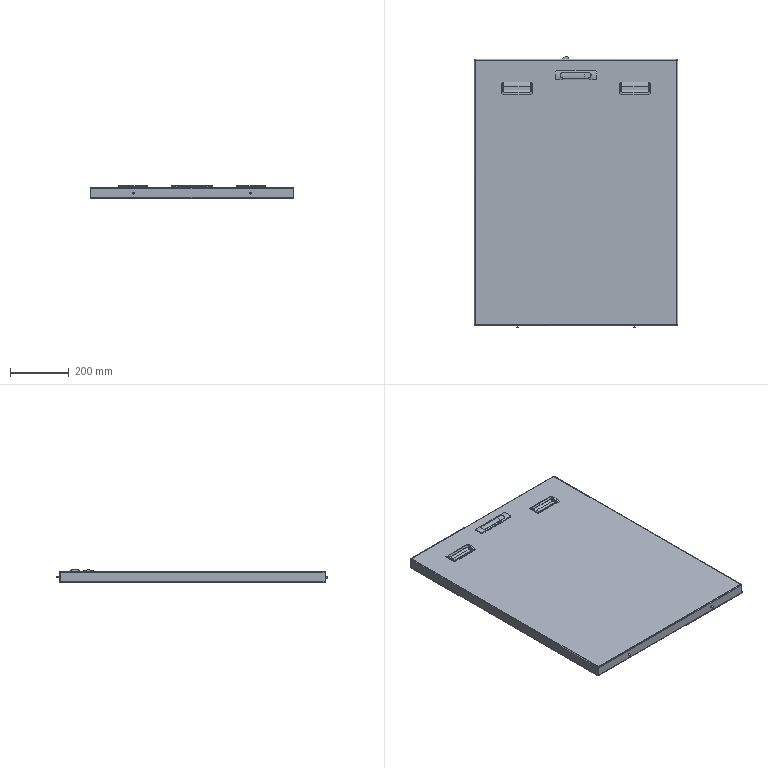Part | SolidWorks | 6 solids | 488 faces | box 695 x 928.5 x 44 mm | volume 1328508 mm3 | plane 222 | cylinder 188 | spline 46 | cone 26 | torus 6 | commonest cylinder face diameters 10 x27 2 x20 8.136 x15 6.6 x12 7 x11 3.242 x8